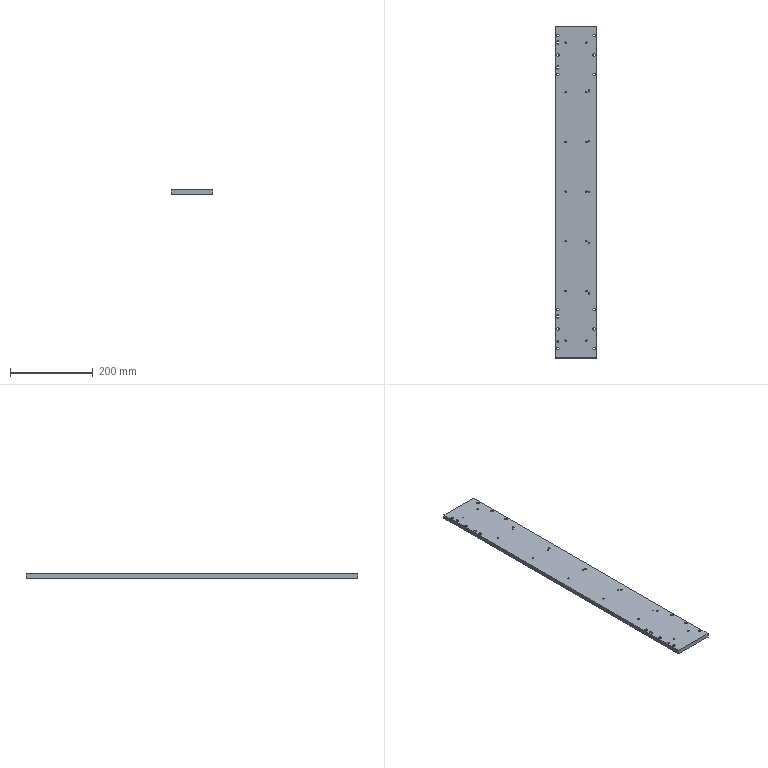Part | STEP file | SynoNew-0304-026 | 1 solid | 86 faces | box 100 x 802 x 10 mm | volume 789361 mm3 | cylinder 56 | plane 24 | cone 6 | commonest cylinder face diameters 3.242 x14 6.6 x12 11 x12 4 x7 3.2 x6 4.2 x5